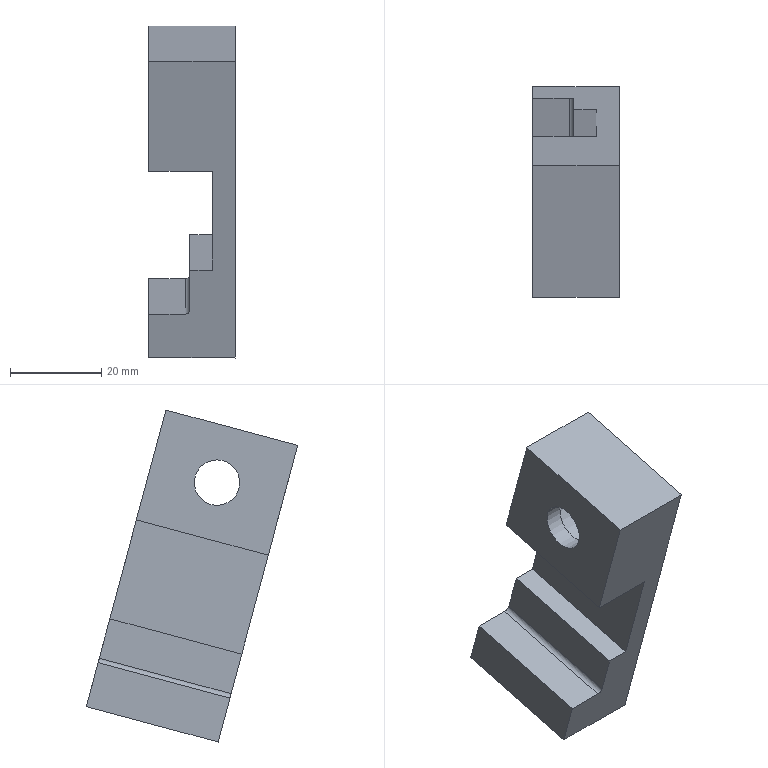Part | NX | features solid 2 | 1 solid | 16 faces | box 19 x 46.448 x 72.965 mm | volume 22409 mm3 | plane 13 | cylinder 3 | commonest cylinder face diameters 2 x1 10 x1 17.5 x1
STEP:
#1=CARTESIAN_POINT('',(208.,916.527,-208.963));
#2=VERTEX_POINT('',#1);
#3=CARTESIAN_POINT('',(208.,915.233,-213.793));
#4=DIRECTION('',(1.,0.000000001,-0.000000005));
#5=DIRECTION('',(0.000000005,0.2588,0.9659));
#6=AXIS2_PLACEMENT_3D('',#3,#4,#5);
#7=CIRCLE('',#6,5.);
#8=EDGE_CURVE('',#2,#2,#7,.T.);
#9=ORIENTED_EDGE('',*,*,#8,.T.);
#10=EDGE_LOOP('',(#9));
#11=FACE_BOUND('',#10,.T.);
#12=CARTESIAN_POINT('',(208.,903.98,-229.749));
#13=VERTEX_POINT('',#12);
#14=CARTESIAN_POINT('',(208.,897.509,-205.601));
#15=VERTEX_POINT('',#14);
#16=CARTESIAN_POINT('',(208.,903.98,-229.749));
#17=DIRECTION('',(0.000000006,-0.2588,0.9659));
#18=VECTOR('',#17,1000.);
#19=LINE('',#16,#18);
#20=EDGE_CURVE('',#13,#15,#19,.T.);
#21=ORIENTED_EDGE('',*,*,#20,.T.);
#22=CARTESIAN_POINT('',(208.,926.487,-197.836));
#23=VERTEX_POINT('',#22);
#24=CARTESIAN_POINT('',(208.,926.487,-197.836));
#25=DIRECTION('',(0.,-0.9659,-0.2588));
#26=VECTOR('',#25,1000.);
#27=LINE('',#24,#26);
#28=EDGE_CURVE('',#23,#15,#27,.T.);
#29=ORIENTED_EDGE('',*,*,#28,.F.);
#30=CARTESIAN_POINT('',(208.,932.957,-221.985));
#31=VERTEX_POINT('',#30);
#32=CARTESIAN_POINT('',(208.,932.957,-221.985));
#33=DIRECTION('',(0.000000006,-0.2588,0.9659));
#34=VECTOR('',#33,1000.);
#35=LINE('',#32,#34);
#36=EDGE_CURVE('',#31,#23,#35,.T.);
#37=ORIENTED_EDGE('',*,*,#36,.F.);
#38=CARTESIAN_POINT('',(208.,932.957,-221.985));
#39=DIRECTION('',(0.,-0.9659,-0.2588));
#40=VECTOR('',#39,1000.);
#41=LINE('',#38,#40);
#42=EDGE_CURVE('',#31,#13,#41,.T.);
#43=ORIENTED_EDGE('',*,*,#42,.T.);
#44=EDGE_LOOP('',(#21,#29,#37,#43));
#45=FACE_BOUND('',#44,.T.);
#46=CARTESIAN_POINT('',(208.,932.957,-221.985));
#47=DIRECTION('',(-1.,-0.000000001,0.000000005));
#48=DIRECTION('',(0.000000005,0.2588,0.9659));
#49=AXIS2_PLACEMENT_3D('',#46,#47,#48);
#50=PLANE('',#49);
#51=ADVANCED_FACE('',(#11,#45),#50,.T.);
#52=CARTESIAN_POINT('',(227.,897.509,-205.601));
#53=VERTEX_POINT('',#52);
#54=CARTESIAN_POINT('',(227.,897.509,-205.601));
#55=DIRECTION('',(-1.,-0.000000001,0.000000005));
#56=VECTOR('',#55,1000.);
#57=LINE('',#54,#56);
#58=EDGE_CURVE('',#53,#15,#57,.T.);
#59=ORIENTED_EDGE('',*,*,#58,.F.);
#60=CARTESIAN_POINT('',(227.,926.487,-197.836));
#61=VERTEX_POINT('',#60);
#62=CARTESIAN_POINT('',(227.,926.487,-197.836));
#63=DIRECTION('',(0.,-0.9659,-0.2588));
#64=VECTOR('',#63,1000.);
#65=LINE('',#62,#64);
#66=EDGE_CURVE('',#61,#53,#65,.T.);
#67=ORIENTED_EDGE('',*,*,#66,.F.);
#68=CARTESIAN_POINT('',(227.,926.487,-197.836));
#69=DIRECTION('',(-1.,-0.000000001,0.000000005));
#70=VECTOR('',#69,1000.);
#71=LINE('',#68,#70);
#72=EDGE_CURVE('',#61,#23,#71,.T.);
#73=ORIENTED_EDGE('',*,*,#72,.T.);
#74=ORIENTED_EDGE('',*,*,#28,.T.);
#75=EDGE_LOOP('',(#59,#67,#73,#74));
#76=FACE_BOUND('',#75,.T.);
#77=CARTESIAN_POINT('',(227.,926.487,-197.836));
#78=DIRECTION('',(-0.000000006,0.2588,-0.9659));
#79=DIRECTION('',(0.,-0.9659,-0.2588));
#80=AXIS2_PLACEMENT_3D('',#77,#78,#79);
#81=PLANE('',#80);
#82=ADVANCED_FACE('',(#76),#81,.F.);
#83=CARTESIAN_POINT('',(227.,912.969,-222.245));
#84=VERTEX_POINT('',#83);
#85=CARTESIAN_POINT('',(227.,915.233,-213.793));
#86=DIRECTION('',(-1.,0.000000001,-0.000000005));
#87=DIRECTION('',(0.000000004,-0.2588,-0.9659));
#88=AXIS2_PLACEMENT_3D('',#85,#86,#87);
#89=CIRCLE('',#88,8.75);
#90=EDGE_CURVE('',#84,#84,#89,.T.);
#91=ORIENTED_EDGE('',*,*,#90,.T.);
#92=EDGE_LOOP('',(#91));
#93=FACE_BOUND('',#92,.T.);
#94=CARTESIAN_POINT('',(227.,914.979,-270.801));
#95=VERTEX_POINT('',#94);
#96=CARTESIAN_POINT('',(227.,909.803,-251.482));
#97=DIRECTION('',(0.000000005,0.2588,-0.9659));
#98=VECTOR('',#97,1000.);
#99=LINE('',#96,#98);
#100=EDGE_CURVE('',#53,#95,#99,.T.);
#101=ORIENTED_EDGE('',*,*,#100,.T.);
#102=CARTESIAN_POINT('',(227.,943.957,-263.036));
#103=VERTEX_POINT('',#102);
#104=CARTESIAN_POINT('',(227.,943.957,-263.036));
#105=DIRECTION('',(0.,-0.9659,-0.2588));
#106=VECTOR('',#105,1000.);
#107=LINE('',#104,#106);
#108=EDGE_CURVE('',#103,#95,#107,.T.);
#109=ORIENTED_EDGE('',*,*,#108,.F.);
#110=CARTESIAN_POINT('',(227.,936.193,-234.059));
#111=DIRECTION('',(-0.000000005,-0.2588,0.9659));
#112=VECTOR('',#111,1000.);
#113=LINE('',#110,#112);
#114=EDGE_CURVE('',#103,#61,#113,.T.);
#115=ORIENTED_EDGE('',*,*,#114,.T.);
#116=ORIENTED_EDGE('',*,*,#66,.T.);
#117=EDGE_LOOP('',(#101,#109,#115,#116));
#118=FACE_BOUND('',#117,.T.);
#119=CARTESIAN_POINT('',(227.,938.781,-243.718));
#120=DIRECTION('',(1.,-0.000000001,0.000000005));
#121=DIRECTION('',(0.000000004,-0.2588,-0.9659));
#122=AXIS2_PLACEMENT_3D('',#119,#120,#121);
#123=PLANE('',#122);
#124=ADVANCED_FACE('',(#93,#118),#123,.T.);
#125=CARTESIAN_POINT('',(208.,914.979,-270.801));
#126=VERTEX_POINT('',#125);
#127=CARTESIAN_POINT('',(208.,914.979,-270.801));
#128=DIRECTION('',(1.,0.000000001,-0.000000005));
#129=VECTOR('',#128,1000.);
#130=LINE('',#127,#129);
#131=EDGE_CURVE('',#126,#95,#130,.T.);
#132=ORIENTED_EDGE('',*,*,#131,.F.);
#133=CARTESIAN_POINT('',(208.,943.957,-263.036));
#134=VERTEX_POINT('',#133);
#135=CARTESIAN_POINT('',(208.,943.957,-263.036));
#136=DIRECTION('',(0.,-0.9659,-0.2588));
#137=VECTOR('',#136,1000.);
#138=LINE('',#135,#137);
#139=EDGE_CURVE('',#134,#126,#138,.T.);
#140=ORIENTED_EDGE('',*,*,#139,.F.);
#141=CARTESIAN_POINT('',(208.,943.957,-263.036));
#142=DIRECTION('',(1.,0.000000001,-0.000000005));
#143=VECTOR('',#142,1000.);
#144=LINE('',#141,#143);
#145=EDGE_CURVE('',#134,#103,#144,.T.);
#146=ORIENTED_EDGE('',*,*,#145,.T.);
#147=ORIENTED_EDGE('',*,*,#108,.T.);
#148=EDGE_LOOP('',(#132,#140,#146,#147));
#149=FACE_BOUND('',#148,.T.);
#150=CARTESIAN_POINT('',(208.,943.957,-263.036));
#151=DIRECTION('',(0.000000006,-0.2588,0.9659));
#152=DIRECTION('',(0.,0.9659,0.2588));
#153=AXIS2_PLACEMENT_3D('',#150,#151,#152);
#154=PLANE('',#153);
#155=ADVANCED_FACE('',(#149),#154,.F.);
#156=CARTESIAN_POINT('',(208.,912.391,-261.142));
#157=VERTEX_POINT('',#156);
#158=CARTESIAN_POINT('',(208.,912.391,-261.142));
#159=DIRECTION('',(0.000000005,0.2588,-0.9659));
#160=VECTOR('',#159,1000.);
#161=LINE('',#158,#160);
#162=EDGE_CURVE('',#157,#126,#161,.T.);
#163=ORIENTED_EDGE('',*,*,#162,.F.);
#164=CARTESIAN_POINT('',(208.,941.369,-253.377));
#165=VERTEX_POINT('',#164);
#166=CARTESIAN_POINT('',(208.,941.369,-253.377));
#167=DIRECTION('',(0.,-0.9659,-0.2588));
#168=VECTOR('',#167,1000.);
#169=LINE('',#166,#168);
#170=EDGE_CURVE('',#165,#157,#169,.T.);
#171=ORIENTED_EDGE('',*,*,#170,.F.);
#172=CARTESIAN_POINT('',(208.,941.369,-253.377));
#173=DIRECTION('',(0.000000005,0.2588,-0.9659));
#174=VECTOR('',#173,1000.);
#175=LINE('',#172,#174);
#176=EDGE_CURVE('',#165,#134,#175,.T.);
#177=ORIENTED_EDGE('',*,*,#176,.T.);
#178=ORIENTED_EDGE('',*,*,#139,.T.);
#179=EDGE_LOOP('',(#163,#171,#177,#178));
#180=FACE_BOUND('',#179,.T.);
#181=CARTESIAN_POINT('',(208.,941.369,-253.377));
#182=DIRECTION('',(1.,-0.000000001,0.000000005));
#183=DIRECTION('',(0.000000004,-0.2588,-0.9659));
#184=AXIS2_PLACEMENT_3D('',#181,#182,#183);
#185=PLANE('',#184);
#186=ADVANCED_FACE('',(#180),#185,.F.);
#187=CARTESIAN_POINT('',(216.,912.391,-261.142));
#188=VERTEX_POINT('',#187);
#189=CARTESIAN_POINT('',(215.,912.391,-261.142));
#190=DIRECTION('',(1.,-0.000000005,0.000000017));
#191=VECTOR('',#190,1000.);
#192=LINE('',#189,#191);
#193=EDGE_CURVE('',#157,#188,#192,.T.);
#194=ORIENTED_EDGE('',*,*,#193,.T.);
#195=CARTESIAN_POINT('',(216.,941.369,-253.377));
#196=VERTEX_POINT('',#195);
#197=CARTESIAN_POINT('',(216.,941.369,-253.377));
#198=DIRECTION('',(0.,-0.9659,-0.2588));
#199=VECTOR('',#198,1000.);
#200=LINE('',#197,#199);
#201=EDGE_CURVE('',#196,#188,#200,.T.);
#202=ORIENTED_EDGE('',*,*,#201,.F.);
#203=CARTESIAN_POINT('',(208.,941.369,-253.377));
#204=DIRECTION('',(1.,-0.000000005,0.000000017));
#205=VECTOR('',#204,1000.);
#206=LINE('',#203,#205);
#207=EDGE_CURVE('',#165,#196,#206,.T.);
#208=ORIENTED_EDGE('',*,*,#207,.F.);
#209=ORIENTED_EDGE('',*,*,#170,.T.);
#210=EDGE_LOOP('',(#194,#202,#208,#209));
#211=FACE_BOUND('',#210,.T.);
#212=CARTESIAN_POINT('',(215.,941.369,-253.377));
#213=DIRECTION('',(-0.000000018,-0.2588,0.9659));
#214=DIRECTION('',(0.,0.9659,0.2588));
#215=AXIS2_PLACEMENT_3D('',#212,#213,#214);
#216=PLANE('',#215);
#217=ADVANCED_FACE('',(#211),#216,.T.);
#218=CARTESIAN_POINT('',(217.,912.132,-260.176));
#219=VERTEX_POINT('',#218);
#220=CARTESIAN_POINT('',(216.,912.132,-260.176));
#221=DIRECTION('',(0.,0.9659,0.2588));
#222=DIRECTION('',(-0.866,-0.1294,0.483));
#223=AXIS2_PLACEMENT_3D('',#220,#221,#222);
#224=CIRCLE('',#223,1.);
#225=EDGE_CURVE('',#219,#188,#224,.T.);
#226=ORIENTED_EDGE('',*,*,#225,.F.);
#227=CARTESIAN_POINT('',(217.,941.11,-252.411));
#228=VERTEX_POINT('',#227);
#229=CARTESIAN_POINT('',(217.,941.11,-252.411));
#230=DIRECTION('',(0.,-0.9659,-0.2588));
#231=VECTOR('',#230,1000.);
#232=LINE('',#229,#231);
#233=EDGE_CURVE('',#228,#219,#232,.T.);
#234=ORIENTED_EDGE('',*,*,#233,.F.);
#235=CARTESIAN_POINT('',(216.,941.11,-252.411));
#236=DIRECTION('',(0.,0.9659,0.2588));
#237=DIRECTION('',(-0.866,-0.1294,0.483));
#238=AXIS2_PLACEMENT_3D('',#235,#236,#237);
#239=CIRCLE('',#238,1.);
#240=EDGE_CURVE('',#228,#196,#239,.T.);
#241=ORIENTED_EDGE('',*,*,#240,.T.);
#242=ORIENTED_EDGE('',*,*,#201,.T.);
#243=EDGE_LOOP('',(#226,#234,#241,#242));
#244=FACE_BOUND('',#243,.T.);
#245=CARTESIAN_POINT('',(216.,941.11,-252.411));
#246=DIRECTION('',(0.,-0.9659,-0.2588));
#247=DIRECTION('',(0.,-0.2588,0.9659));
#248=AXIS2_PLACEMENT_3D('',#245,#246,#247);
#249=CYLINDRICAL_SURFACE('',#248,1.);
#250=ADVANCED_FACE('',(#244),#249,.F.);
#251=CARTESIAN_POINT('',(217.,909.803,-251.482));
#252=VERTEX_POINT('',#251);
#253=CARTESIAN_POINT('',(217.,909.803,-251.482));
#254=DIRECTION('',(-0.000000017,0.2588,-0.9659));
#255=VECTOR('',#254,1000.);
#256=LINE('',#253,#255);
#257=EDGE_CURVE('',#252,#219,#256,.T.);
#258=ORIENTED_EDGE('',*,*,#257,.F.);
#259=CARTESIAN_POINT('',(217.,938.781,-243.718));
#260=VERTEX_POINT('',#259);
#261=CARTESIAN_POINT('',(217.,938.781,-243.718));
#262=DIRECTION('',(0.,-0.9659,-0.2588));
#263=VECTOR('',#262,1000.);
#264=LINE('',#261,#263);
#265=EDGE_CURVE('',#260,#252,#264,.T.);
#266=ORIENTED_EDGE('',*,*,#265,.F.);
#267=CARTESIAN_POINT('',(217.,938.781,-243.718));
#268=DIRECTION('',(-0.000000017,0.2588,-0.9659));
#269=VECTOR('',#268,1000.);
#270=LINE('',#267,#269);
#271=EDGE_CURVE('',#260,#228,#270,.T.);
#272=ORIENTED_EDGE('',*,*,#271,.T.);
#273=ORIENTED_EDGE('',*,*,#233,.T.);
#274=EDGE_LOOP('',(#258,#266,#272,#273));
#275=FACE_BOUND('',#274,.T.);
#276=CARTESIAN_POINT('',(217.,938.781,-243.718));
#277=DIRECTION('',(1.,0.000000004,-0.000000017));
#278=DIRECTION('',(-0.000000015,-0.2588,-0.9659));
#279=AXIS2_PLACEMENT_3D('',#276,#277,#278);
#280=PLANE('',#279);
#281=ADVANCED_FACE('',(#275),#280,.F.);
#282=CARTESIAN_POINT('',(222.,909.803,-251.482));
#283=VERTEX_POINT('',#282);
#284=CARTESIAN_POINT('',(222.,909.803,-251.482));
#285=DIRECTION('',(-1.,0.000000003,-0.000000012));
#286=VECTOR('',#285,1000.);
#287=LINE('',#284,#286);
#288=EDGE_CURVE('',#283,#252,#287,.T.);
#289=ORIENTED_EDGE('',*,*,#288,.F.);
#290=CARTESIAN_POINT('',(222.,938.781,-243.718));
#291=VERTEX_POINT('',#290);
#292=CARTESIAN_POINT('',(222.,938.781,-243.718));
#293=DIRECTION('',(0.,-0.9659,-0.2588));
#294=VECTOR('',#293,1000.);
#295=LINE('',#292,#294);
#296=EDGE_CURVE('',#291,#283,#295,.T.);
#297=ORIENTED_EDGE('',*,*,#296,.F.);
#298=CARTESIAN_POINT('',(222.,938.781,-243.718));
#299=DIRECTION('',(-1.,0.000000003,-0.000000012));
#300=VECTOR('',#299,1000.);
#301=LINE('',#298,#300);
#302=EDGE_CURVE('',#291,#260,#301,.T.);
#303=ORIENTED_EDGE('',*,*,#302,.T.);
#304=ORIENTED_EDGE('',*,*,#265,.T.);
#305=EDGE_LOOP('',(#289,#297,#303,#304));
#306=FACE_BOUND('',#305,.T.);
#307=CARTESIAN_POINT('',(222.,938.781,-243.718));
#308=DIRECTION('',(0.000000012,0.2588,-0.9659));
#309=DIRECTION('',(0.,-0.9659,-0.2588));
#310=AXIS2_PLACEMENT_3D('',#307,#308,#309);
#311=PLANE('',#310);
#312=ADVANCED_FACE('',(#306),#311,.F.);
#313=CARTESIAN_POINT('',(222.,903.98,-229.749));
#314=VERTEX_POINT('',#313);
#315=CARTESIAN_POINT('',(222.,903.98,-229.749));
#316=DIRECTION('',(0.000000005,0.2588,-0.9659));
#317=VECTOR('',#316,1000.);
#318=LINE('',#315,#317);
#319=EDGE_CURVE('',#314,#283,#318,.T.);
#320=ORIENTED_EDGE('',*,*,#319,.F.);
#321=CARTESIAN_POINT('',(222.,932.957,-221.985));
#322=VERTEX_POINT('',#321);
#323=CARTESIAN_POINT('',(222.,932.957,-221.985));
#324=DIRECTION('',(0.,-0.9659,-0.2588));
#325=VECTOR('',#324,1000.);
#326=LINE('',#323,#325);
#327=EDGE_CURVE('',#322,#314,#326,.T.);
#328=ORIENTED_EDGE('',*,*,#327,.F.);
#329=CARTESIAN_POINT('',(222.,936.193,-234.059));
#330=DIRECTION('',(0.000000005,0.2588,-0.9659));
#331=VECTOR('',#330,1000.);
#332=LINE('',#329,#331);
#333=EDGE_CURVE('',#322,#291,#332,.T.);
#334=ORIENTED_EDGE('',*,*,#333,.T.);
#335=ORIENTED_EDGE('',*,*,#296,.T.);
#336=EDGE_LOOP('',(#320,#328,#334,#335));
#337=FACE_BOUND('',#336,.T.);
#338=CARTESIAN_POINT('',(222.,932.957,-221.985));
#339=DIRECTION('',(1.,-0.000000001,0.000000005));
#340=DIRECTION('',(0.000000004,-0.2588,-0.9659));
#341=AXIS2_PLACEMENT_3D('',#338,#339,#340);
#342=PLANE('',#341);
#343=ADVANCED_FACE('',(#337),#342,.F.);
#344=CARTESIAN_POINT('',(222.,903.98,-229.749));
#345=DIRECTION('',(-1.,-0.000000001,0.000000005));
#346=VECTOR('',#345,1000.);
#347=LINE('',#344,#346);
#348=EDGE_CURVE('',#314,#13,#347,.T.);
#349=ORIENTED_EDGE('',*,*,#348,.T.);
#350=ORIENTED_EDGE('',*,*,#42,.F.);
#351=CARTESIAN_POINT('',(222.,932.957,-221.985));
#352=DIRECTION('',(-1.,-0.000000001,0.000000005));
#353=VECTOR('',#352,1000.);
#354=LINE('',#351,#353);
#355=EDGE_CURVE('',#322,#31,#354,.T.);
#356=ORIENTED_EDGE('',*,*,#355,.F.);
#357=ORIENTED_EDGE('',*,*,#327,.T.);
#358=EDGE_LOOP('',(#349,#350,#356,#357));
#359=FACE_BOUND('',#358,.T.);
#360=CARTESIAN_POINT('',(222.,932.957,-221.985));
#361=DIRECTION('',(-0.000000006,0.2588,-0.9659));
#362=DIRECTION('',(0.,-0.9659,-0.2588));
#363=AXIS2_PLACEMENT_3D('',#360,#361,#362);
#364=PLANE('',#363);
#365=ADVANCED_FACE('',(#359),#364,.T.);
#366=ORIENTED_EDGE('',*,*,#36,.T.);
#367=ORIENTED_EDGE('',*,*,#72,.F.);
#368=ORIENTED_EDGE('',*,*,#114,.F.);
#369=ORIENTED_EDGE('',*,*,#145,.F.);
#370=ORIENTED_EDGE('',*,*,#176,.F.);
#371=ORIENTED_EDGE('',*,*,#207,.T.);
#372=ORIENTED_EDGE('',*,*,#240,.F.);
#373=ORIENTED_EDGE('',*,*,#271,.F.);
#374=ORIENTED_EDGE('',*,*,#302,.F.);
#375=ORIENTED_EDGE('',*,*,#333,.F.);
#376=ORIENTED_EDGE('',*,*,#355,.T.);
#377=EDGE_LOOP('',(#366,#367,#368,#369,#370,#371,#372,#373,#374,#375,#376));
#378=FACE_BOUND('',#377,.T.);
#379=CARTESIAN_POINT('',(216.,941.11,-252.411));
#380=DIRECTION('',(0.,-0.9659,-0.2588));
#381=DIRECTION('',(0.,-0.2588,0.9659));
#382=AXIS2_PLACEMENT_3D('',#379,#380,#381);
#383=PLANE('',#382);
#384=ADVANCED_FACE('',(#378),#383,.F.);
#385=ORIENTED_EDGE('',*,*,#20,.F.);
#386=ORIENTED_EDGE('',*,*,#348,.F.);
#387=ORIENTED_EDGE('',*,*,#319,.T.);
#388=ORIENTED_EDGE('',*,*,#288,.T.);
#389=ORIENTED_EDGE('',*,*,#257,.T.);
#390=ORIENTED_EDGE('',*,*,#225,.T.);
#391=ORIENTED_EDGE('',*,*,#193,.F.);
#392=ORIENTED_EDGE('',*,*,#162,.T.);
#393=ORIENTED_EDGE('',*,*,#131,.T.);
#394=ORIENTED_EDGE('',*,*,#100,.F.);
#395=ORIENTED_EDGE('',*,*,#58,.T.);
#396=EDGE_LOOP('',(#385,#386,#387,#388,#389,#390,#391,#392,#393,#394,#395));
#397=FACE_BOUND('',#396,.T.);
#398=CARTESIAN_POINT('',(216.,912.132,-260.176));
#399=DIRECTION('',(0.,-0.9659,-0.2588));
#400=DIRECTION('',(0.,-0.2588,0.9659));
#401=AXIS2_PLACEMENT_3D('',#398,#399,#400);
#402=PLANE('',#401);
#403=ADVANCED_FACE('',(#397),#402,.T.);
#404=CARTESIAN_POINT('',(212.,912.969,-222.245));
#405=VERTEX_POINT('',#404);
#406=CARTESIAN_POINT('',(212.,915.233,-213.793));
#407=DIRECTION('',(-1.,0.000000001,-0.000000005));
#408=DIRECTION('',(0.000000004,-0.2588,-0.9659));
#409=AXIS2_PLACEMENT_3D('',#406,#407,#408);
#410=CIRCLE('',#409,8.75);
#411=EDGE_CURVE('',#405,#405,#410,.T.);
#412=ORIENTED_EDGE('',*,*,#411,.T.);
#413=EDGE_LOOP('',(#412));
#414=FACE_BOUND('',#413,.T.);
#415=ORIENTED_EDGE('',*,*,#90,.F.);
#416=EDGE_LOOP('',(#415));
#417=FACE_BOUND('',#416,.T.);
#418=CARTESIAN_POINT('',(212.,915.233,-213.793));
#419=DIRECTION('',(1.,-0.000000001,0.000000005));
#420=DIRECTION('',(0.000000004,-0.2588,-0.9659));
#421=AXIS2_PLACEMENT_3D('',#418,#419,#420);
#422=CYLINDRICAL_SURFACE('',#421,8.75);
#423=ADVANCED_FACE('',(#414,#417),#422,.F.);
#424=CARTESIAN_POINT('',(212.,913.939,-218.622));
#425=VERTEX_POINT('',#424);
#426=CARTESIAN_POINT('',(212.,915.233,-213.793));
#427=DIRECTION('',(-1.,0.000000001,-0.000000005));
#428=DIRECTION('',(0.000000004,-0.2588,-0.9659));
#429=AXIS2_PLACEMENT_3D('',#426,#427,#428);
#430=CIRCLE('',#429,5.);
#431=EDGE_CURVE('',#425,#425,#430,.T.);
#432=ORIENTED_EDGE('',*,*,#431,.T.);
#433=EDGE_LOOP('',(#432));
#434=FACE_BOUND('',#433,.T.);
#435=ORIENTED_EDGE('',*,*,#411,.F.);
#436=EDGE_LOOP('',(#435));
#437=FACE_BOUND('',#436,.T.);
#438=CARTESIAN_POINT('',(212.,915.233,-213.793));
#439=DIRECTION('',(1.,-0.000000001,0.000000005));
#440=DIRECTION('',(0.000000004,-0.2588,-0.9659));
#441=AXIS2_PLACEMENT_3D('',#438,#439,#440);
#442=PLANE('',#441);
#443=ADVANCED_FACE('',(#434,#437),#442,.T.);
#444=ORIENTED_EDGE('',*,*,#8,.F.);
#445=EDGE_LOOP('',(#444));
#446=FACE_BOUND('',#445,.T.);
#447=ORIENTED_EDGE('',*,*,#431,.F.);
#448=EDGE_LOOP('',(#447));
#449=FACE_BOUND('',#448,.T.);
#450=CARTESIAN_POINT('',(190.,915.233,-213.793));
#451=DIRECTION('',(1.,-0.000000001,0.000000005));
#452=DIRECTION('',(0.000000004,-0.2588,-0.9659));
#453=AXIS2_PLACEMENT_3D('',#450,#451,#452);
#454=CYLINDRICAL_SURFACE('',#453,5.);
#455=ADVANCED_FACE('',(#446,#449),#454,.F.);
#456=CLOSED_SHELL('',(#51,#82,#124,#155,#186,#217,#250,#281,#312,#343,#365,#384,#403,#423,#443,#455));
#457=MANIFOLD_SOLID_BREP('',#456);
#458=(LENGTH_UNIT()NAMED_UNIT(*)SI_UNIT(.MILLI.,.METRE.));
#459=UNCERTAINTY_MEASURE_WITH_UNIT(LENGTH_MEASURE(0.00001),#458,'','');
#460=(NAMED_UNIT(*)PLANE_ANGLE_UNIT()SI_UNIT($,.RADIAN.));
#461=(NAMED_UNIT(*)SI_UNIT($,.STERADIAN.)SOLID_ANGLE_UNIT());
#462=(GEOMETRIC_REPRESENTATION_CONTEXT(3)GLOBAL_UNCERTAINTY_ASSIGNED_CONTEXT((#459))GLOBAL_UNIT_ASSIGNED_CONTEXT((#458,#460,#461))REPRESENTATION_CONTEXT('',''));
#463=ADVANCED_BREP_SHAPE_REPRESENTATION('',(#457),#462);